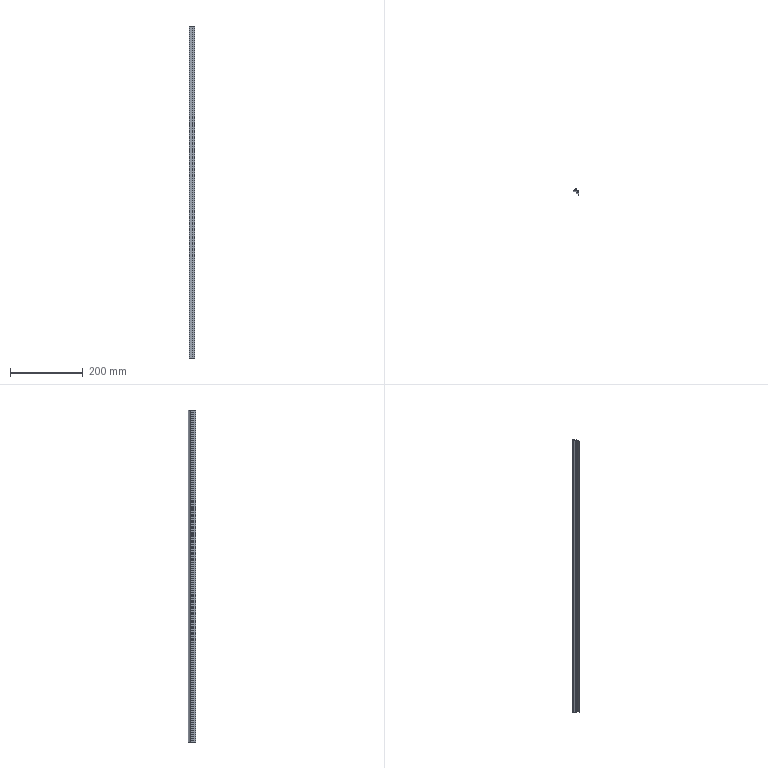Part | SolidWorks | features BaseBody 1, ICE 1, MoveFace 1 | 1 solid | 27 faces | box 14 x 20.3 x 915 mm | volume 46588 mm3 | plane 20 | cylinder 7 | commonest cylinder face diameters 0.387 x2 0.8 x2 0.4 x1 20 x1 22 x1
STEP:
#1=CARTESIAN_POINT('',(-5.304,-0.625,200.));
#2=VERTEX_POINT('',#1);
#3=CARTESIAN_POINT('',(-5.449,-0.8125,200.));
#4=VERTEX_POINT('',#3);
#5=CARTESIAN_POINT('',(-5.255,-0.8125,200.));
#6=DIRECTION('',(0.,0.,1.));
#7=DIRECTION('',(-1.,0.,0.));
#8=AXIS2_PLACEMENT_3D('',#5,#6,#7);
#9=CIRCLE('',#8,0.1937);
#10=EDGE_CURVE('',#2,#4,#9,.T.);
#11=ORIENTED_EDGE('',*,*,#10,.T.);
#12=CARTESIAN_POINT('',(-5.449,-0.8125,-715.));
#13=VERTEX_POINT('',#12);
#14=CARTESIAN_POINT('',(-5.449,-0.8125,230.));
#15=DIRECTION('',(0.,0.,-1.));
#16=VECTOR('',#15,1000.);
#17=LINE('',#14,#16);
#18=EDGE_CURVE('',#4,#13,#17,.T.);
#19=ORIENTED_EDGE('',*,*,#18,.T.);
#20=CARTESIAN_POINT('',(-5.304,-0.625,-715.));
#21=VERTEX_POINT('',#20);
#22=CARTESIAN_POINT('',(-5.255,-0.8125,-715.));
#23=DIRECTION('',(0.,0.,-1.));
#24=DIRECTION('',(1.,0.,0.));
#25=AXIS2_PLACEMENT_3D('',#22,#23,#24);
#26=CIRCLE('',#25,0.1937);
#27=EDGE_CURVE('',#13,#21,#26,.T.);
#28=ORIENTED_EDGE('',*,*,#27,.T.);
#29=CARTESIAN_POINT('',(-5.304,-0.625,230.));
#30=DIRECTION('',(0.,0.,-1.));
#31=VECTOR('',#30,1000.);
#32=LINE('',#29,#31);
#33=EDGE_CURVE('',#2,#21,#32,.T.);
#34=ORIENTED_EDGE('',*,*,#33,.F.);
#35=EDGE_LOOP('',(#11,#19,#28,#34));
#36=FACE_OUTER_BOUND('',#35,.T.);
#37=CARTESIAN_POINT('',(-5.255,-0.8125,230.));
#38=DIRECTION('',(0.,0.,-1.));
#39=DIRECTION('',(-1.,0.,0.));
#40=AXIS2_PLACEMENT_3D('',#37,#38,#39);
#41=CYLINDRICAL_SURFACE('',#40,0.1937);
#42=ADVANCED_FACE('',(#36),#41,.F.);
#43=CARTESIAN_POINT('',(5.,-1.,-715.));
#44=VERTEX_POINT('',#43);
#45=CARTESIAN_POINT('',(5.,-14.3,-715.));
#46=VERTEX_POINT('',#45);
#47=CARTESIAN_POINT('',(5.,29.623,-715.));
#48=DIRECTION('',(0.,-1.,0.));
#49=VECTOR('',#48,1000.);
#50=LINE('',#47,#49);
#51=EDGE_CURVE('',#44,#46,#50,.T.);
#52=ORIENTED_EDGE('',*,*,#51,.F.);
#53=CARTESIAN_POINT('',(5.,-1.,200.));
#54=VERTEX_POINT('',#53);
#55=CARTESIAN_POINT('',(5.,-1.,230.));
#56=DIRECTION('',(0.,0.,-1.));
#57=VECTOR('',#56,1000.);
#58=LINE('',#55,#57);
#59=EDGE_CURVE('',#54,#44,#58,.T.);
#60=ORIENTED_EDGE('',*,*,#59,.F.);
#61=CARTESIAN_POINT('',(5.,-14.3,200.));
#62=VERTEX_POINT('',#61);
#63=CARTESIAN_POINT('',(5.,-14.3,200.));
#64=DIRECTION('',(0.,1.,0.));
#65=VECTOR('',#64,1000.);
#66=LINE('',#63,#65);
#67=EDGE_CURVE('',#62,#54,#66,.T.);
#68=ORIENTED_EDGE('',*,*,#67,.F.);
#69=CARTESIAN_POINT('',(5.,-14.3,230.));
#70=DIRECTION('',(0.,0.,1.));
#71=VECTOR('',#70,1000.);
#72=LINE('',#69,#71);
#73=EDGE_CURVE('',#46,#62,#72,.T.);
#74=ORIENTED_EDGE('',*,*,#73,.F.);
#75=EDGE_LOOP('',(#52,#60,#68,#74));
#76=FACE_OUTER_BOUND('',#75,.T.);
#77=CARTESIAN_POINT('',(5.,-14.3,230.));
#78=DIRECTION('',(-1.,0.,0.));
#79=DIRECTION('',(0.,0.,1.));
#80=AXIS2_PLACEMENT_3D('',#77,#78,#79);
#81=PLANE('',#80);
#82=ADVANCED_FACE('',(#76),#81,.F.);
#83=CARTESIAN_POINT('',(-9.,-2.,-715.));
#84=VERTEX_POINT('',#83);
#85=CARTESIAN_POINT('',(-9.,-2.,200.));
#86=VERTEX_POINT('',#85);
#87=CARTESIAN_POINT('',(-9.,-2.,230.));
#88=DIRECTION('',(0.,0.,1.));
#89=VECTOR('',#88,1000.);
#90=LINE('',#87,#89);
#91=EDGE_CURVE('',#84,#86,#90,.T.);
#92=ORIENTED_EDGE('',*,*,#91,.F.);
#93=CARTESIAN_POINT('',(0.9,-2.,-715.));
#94=VERTEX_POINT('',#93);
#95=CARTESIAN_POINT('',(5.,-2.,-715.));
#96=DIRECTION('',(-1.,0.,0.));
#97=VECTOR('',#96,1000.);
#98=LINE('',#95,#97);
#99=EDGE_CURVE('',#94,#84,#98,.T.);
#100=ORIENTED_EDGE('',*,*,#99,.F.);
#101=CARTESIAN_POINT('',(0.9,-2.,200.));
#102=VERTEX_POINT('',#101);
#103=CARTESIAN_POINT('',(0.9,-2.,230.));
#104=DIRECTION('',(0.,0.,-1.));
#105=VECTOR('',#104,1000.);
#106=LINE('',#103,#105);
#107=EDGE_CURVE('',#102,#94,#106,.T.);
#108=ORIENTED_EDGE('',*,*,#107,.F.);
#109=CARTESIAN_POINT('',(5.,-2.,200.));
#110=DIRECTION('',(1.,0.,0.));
#111=VECTOR('',#110,1000.);
#112=LINE('',#109,#111);
#113=EDGE_CURVE('',#86,#102,#112,.T.);
#114=ORIENTED_EDGE('',*,*,#113,.F.);
#115=EDGE_LOOP('',(#92,#100,#108,#114));
#116=FACE_OUTER_BOUND('',#115,.T.);
#117=CARTESIAN_POINT('',(-9.,-2.,230.));
#118=DIRECTION('',(0.,1.,0.));
#119=DIRECTION('',(0.,0.,1.));
#120=AXIS2_PLACEMENT_3D('',#117,#118,#119);
#121=PLANE('',#120);
#122=ADVANCED_FACE('',(#116),#121,.F.);
#123=CARTESIAN_POINT('',(4.,-6.,200.));
#124=VERTEX_POINT('',#123);
#125=CARTESIAN_POINT('',(4.,-3.,200.));
#126=VERTEX_POINT('',#125);
#127=CARTESIAN_POINT('',(4.,29.623,200.));
#128=DIRECTION('',(0.,1.,0.));
#129=VECTOR('',#128,1000.);
#130=LINE('',#127,#129);
#131=EDGE_CURVE('',#124,#126,#130,.T.);
#132=ORIENTED_EDGE('',*,*,#131,.F.);
#133=CARTESIAN_POINT('',(1.,-6.,200.));
#134=VERTEX_POINT('',#133);
#135=CARTESIAN_POINT('',(5.,-6.,200.));
#136=DIRECTION('',(1.,0.,0.));
#137=VECTOR('',#136,1000.);
#138=LINE('',#135,#137);
#139=EDGE_CURVE('',#134,#124,#138,.T.);
#140=ORIENTED_EDGE('',*,*,#139,.F.);
#141=CARTESIAN_POINT('',(1.,-6.7,200.));
#142=VERTEX_POINT('',#141);
#143=CARTESIAN_POINT('',(1.,-6.,200.));
#144=DIRECTION('',(0.,-1.,0.));
#145=VECTOR('',#144,1000.);
#146=LINE('',#143,#145);
#147=EDGE_CURVE('',#134,#142,#146,.T.);
#148=ORIENTED_EDGE('',*,*,#147,.T.);
#149=CARTESIAN_POINT('',(-1.7,-6.7,200.));
#150=VERTEX_POINT('',#149);
#151=CARTESIAN_POINT('',(5.,-6.7,200.));
#152=DIRECTION('',(1.,0.,0.));
#153=VECTOR('',#152,1000.);
#154=LINE('',#151,#153);
#155=EDGE_CURVE('',#150,#142,#154,.T.);
#156=ORIENTED_EDGE('',*,*,#155,.F.);
#157=CARTESIAN_POINT('',(-1.7,-7.7,200.));
#158=VERTEX_POINT('',#157);
#159=CARTESIAN_POINT('',(-1.7,-6.7,200.));
#160=DIRECTION('',(0.,-1.,0.));
#161=VECTOR('',#160,1000.);
#162=LINE('',#159,#161);
#163=EDGE_CURVE('',#150,#158,#162,.T.);
#164=ORIENTED_EDGE('',*,*,#163,.T.);
#165=CARTESIAN_POINT('',(4.,-7.7,200.));
#166=VERTEX_POINT('',#165);
#167=CARTESIAN_POINT('',(5.,-7.7,200.));
#168=DIRECTION('',(-1.,0.,0.));
#169=VECTOR('',#168,1000.);
#170=LINE('',#167,#169);
#171=EDGE_CURVE('',#166,#158,#170,.T.);
#172=ORIENTED_EDGE('',*,*,#171,.F.);
#173=CARTESIAN_POINT('',(4.,-14.3,200.));
#174=VERTEX_POINT('',#173);
#175=CARTESIAN_POINT('',(4.,29.623,200.));
#176=DIRECTION('',(0.,1.,0.));
#177=VECTOR('',#176,1000.);
#178=LINE('',#175,#177);
#179=EDGE_CURVE('',#174,#166,#178,.T.);
#180=ORIENTED_EDGE('',*,*,#179,.F.);
#181=CARTESIAN_POINT('',(5.,-14.3,200.));
#182=DIRECTION('',(-1.,0.,0.));
#183=VECTOR('',#182,1000.);
#184=LINE('',#181,#183);
#185=EDGE_CURVE('',#62,#174,#184,.T.);
#186=ORIENTED_EDGE('',*,*,#185,.F.);
#187=ORIENTED_EDGE('',*,*,#67,.T.);
#188=CARTESIAN_POINT('',(-5.207,-1.,200.));
#189=VERTEX_POINT('',#188);
#190=CARTESIAN_POINT('',(5.,-1.,200.));
#191=DIRECTION('',(1.,0.,0.));
#192=VECTOR('',#191,1000.);
#193=LINE('',#190,#192);
#194=EDGE_CURVE('',#189,#54,#193,.T.);
#195=ORIENTED_EDGE('',*,*,#194,.F.);
#196=CARTESIAN_POINT('',(-5.255,-0.8125,200.));
#197=DIRECTION('',(0.,0.,1.));
#198=DIRECTION('',(-1.,0.,0.));
#199=AXIS2_PLACEMENT_3D('',#196,#197,#198);
#200=CIRCLE('',#199,0.1937);
#201=EDGE_CURVE('',#4,#189,#200,.T.);
#202=ORIENTED_EDGE('',*,*,#201,.F.);
#203=ORIENTED_EDGE('',*,*,#10,.F.);
#204=CARTESIAN_POINT('',(-1.368,3.063,200.));
#205=VERTEX_POINT('',#204);
#206=CARTESIAN_POINT('',(-10.628,9.,200.));
#207=DIRECTION('',(0.,0.,1.));
#208=DIRECTION('',(-1.,0.,0.));
#209=AXIS2_PLACEMENT_3D('',#206,#207,#208);
#210=CIRCLE('',#209,11.);
#211=EDGE_CURVE('',#2,#205,#210,.T.);
#212=ORIENTED_EDGE('',*,*,#211,.T.);
#213=CARTESIAN_POINT('',(-1.,2.955,200.));
#214=VERTEX_POINT('',#213);
#215=CARTESIAN_POINT('',(-1.2,2.955,200.));
#216=DIRECTION('',(0.,0.,1.));
#217=DIRECTION('',(-1.,0.,0.));
#218=AXIS2_PLACEMENT_3D('',#215,#216,#217);
#219=CIRCLE('',#218,0.2);
#220=EDGE_CURVE('',#214,#205,#219,.T.);
#221=ORIENTED_EDGE('',*,*,#220,.F.);
#222=CARTESIAN_POINT('',(-1.,1.5,200.));
#223=VERTEX_POINT('',#222);
#224=CARTESIAN_POINT('',(-1.,2.955,200.));
#225=DIRECTION('',(0.,1.,0.));
#226=VECTOR('',#225,1000.);
#227=LINE('',#224,#226);
#228=EDGE_CURVE('',#223,#214,#227,.T.);
#229=ORIENTED_EDGE('',*,*,#228,.F.);
#230=CARTESIAN_POINT('',(0.,1.5,200.));
#231=VERTEX_POINT('',#230);
#232=CARTESIAN_POINT('',(-1.,1.5,200.));
#233=DIRECTION('',(-1.,0.,0.));
#234=VECTOR('',#233,1000.);
#235=LINE('',#232,#234);
#236=EDGE_CURVE('',#231,#223,#235,.T.);
#237=ORIENTED_EDGE('',*,*,#236,.F.);
#238=CARTESIAN_POINT('',(0.,6.,200.));
#239=VERTEX_POINT('',#238);
#240=CARTESIAN_POINT('',(0.,1.5,200.));
#241=DIRECTION('',(0.,-1.,0.));
#242=VECTOR('',#241,1000.);
#243=LINE('',#240,#242);
#244=EDGE_CURVE('',#239,#231,#243,.T.);
#245=ORIENTED_EDGE('',*,*,#244,.F.);
#246=CARTESIAN_POINT('',(-0.8,6.,200.));
#247=VERTEX_POINT('',#246);
#248=CARTESIAN_POINT('',(0.,6.,200.));
#249=DIRECTION('',(1.,0.,0.));
#250=VECTOR('',#249,1000.);
#251=LINE('',#248,#250);
#252=EDGE_CURVE('',#247,#239,#251,.T.);
#253=ORIENTED_EDGE('',*,*,#252,.F.);
#254=CARTESIAN_POINT('',(-1.178,5.731,200.));
#255=VERTEX_POINT('',#254);
#256=CARTESIAN_POINT('',(-0.8,5.6,200.));
#257=DIRECTION('',(0.,0.,1.));
#258=DIRECTION('',(-1.,0.,0.));
#259=AXIS2_PLACEMENT_3D('',#256,#257,#258);
#260=CIRCLE('',#259,0.4);
#261=EDGE_CURVE('',#247,#255,#260,.T.);
#262=ORIENTED_EDGE('',*,*,#261,.T.);
#263=CARTESIAN_POINT('',(-8.678,-0.8077,200.));
#264=VERTEX_POINT('',#263);
#265=CARTESIAN_POINT('',(-10.628,9.,200.));
#266=DIRECTION('',(0.,0.,1.));
#267=DIRECTION('',(-1.,0.,0.));
#268=AXIS2_PLACEMENT_3D('',#265,#266,#267);
#269=CIRCLE('',#268,10.);
#270=EDGE_CURVE('',#264,#255,#269,.T.);
#271=ORIENTED_EDGE('',*,*,#270,.F.);
#272=CARTESIAN_POINT('',(-9.,-1.2,200.));
#273=VERTEX_POINT('',#272);
#274=CARTESIAN_POINT('',(-8.6,-1.2,200.));
#275=DIRECTION('',(0.,0.,1.));
#276=DIRECTION('',(-1.,0.,0.));
#277=AXIS2_PLACEMENT_3D('',#274,#275,#276);
#278=CIRCLE('',#277,0.4);
#279=EDGE_CURVE('',#264,#273,#278,.T.);
#280=ORIENTED_EDGE('',*,*,#279,.T.);
#281=CARTESIAN_POINT('',(-9.,8.,200.));
#282=DIRECTION('',(0.,-1.,0.));
#283=VECTOR('',#282,1000.);
#284=LINE('',#281,#283);
#285=EDGE_CURVE('',#273,#86,#284,.T.);
#286=ORIENTED_EDGE('',*,*,#285,.T.);
#287=ORIENTED_EDGE('',*,*,#113,.T.);
#288=CARTESIAN_POINT('',(0.9,-3.,200.));
#289=VERTEX_POINT('',#288);
#290=CARTESIAN_POINT('',(0.9,29.623,200.));
#291=DIRECTION('',(0.,1.,0.));
#292=VECTOR('',#291,1000.);
#293=LINE('',#290,#292);
#294=EDGE_CURVE('',#289,#102,#293,.T.);
#295=ORIENTED_EDGE('',*,*,#294,.F.);
#296=CARTESIAN_POINT('',(5.,-3.,200.));
#297=DIRECTION('',(-1.,0.,0.));
#298=VECTOR('',#297,1000.);
#299=LINE('',#296,#298);
#300=EDGE_CURVE('',#126,#289,#299,.T.);
#301=ORIENTED_EDGE('',*,*,#300,.F.);
#302=EDGE_LOOP('',(#132,#140,#148,#156,#164,#172,#180,#186,#187,#195,#202,#203,#212,#221,#229,#237,#245,#253,#262,#271,#280,#286,#287,#295,#301));
#303=FACE_OUTER_BOUND('',#302,.T.);
#304=CARTESIAN_POINT('',(5.,29.623,200.));
#305=DIRECTION('',(0.,0.,-1.));
#306=DIRECTION('',(-1.,0.,0.));
#307=AXIS2_PLACEMENT_3D('',#304,#305,#306);
#308=PLANE('',#307);
#309=ADVANCED_FACE('',(#303),#308,.F.);
#310=ORIENTED_EDGE('',*,*,#185,.T.);
#311=CARTESIAN_POINT('',(4.,-14.3,-715.));
#312=VERTEX_POINT('',#311);
#313=CARTESIAN_POINT('',(4.,-14.3,230.));
#314=DIRECTION('',(0.,0.,1.));
#315=VECTOR('',#314,1000.);
#316=LINE('',#313,#315);
#317=EDGE_CURVE('',#312,#174,#316,.T.);
#318=ORIENTED_EDGE('',*,*,#317,.F.);
#319=CARTESIAN_POINT('',(5.,-14.3,-715.));
#320=DIRECTION('',(-1.,0.,0.));
#321=VECTOR('',#320,1000.);
#322=LINE('',#319,#321);
#323=EDGE_CURVE('',#46,#312,#322,.T.);
#324=ORIENTED_EDGE('',*,*,#323,.F.);
#325=ORIENTED_EDGE('',*,*,#73,.T.);
#326=EDGE_LOOP('',(#310,#318,#324,#325));
#327=FACE_OUTER_BOUND('',#326,.T.);
#328=CARTESIAN_POINT('',(4.,-14.3,230.));
#329=DIRECTION('',(0.,1.,0.));
#330=DIRECTION('',(0.,0.,1.));
#331=AXIS2_PLACEMENT_3D('',#328,#329,#330);
#332=PLANE('',#331);
#333=ADVANCED_FACE('',(#327),#332,.F.);
#334=ORIENTED_EDGE('',*,*,#51,.T.);
#335=ORIENTED_EDGE('',*,*,#323,.T.);
#336=CARTESIAN_POINT('',(4.,-7.7,-715.));
#337=VERTEX_POINT('',#336);
#338=CARTESIAN_POINT('',(4.,-7.7,-715.));
#339=DIRECTION('',(0.,-1.,0.));
#340=VECTOR('',#339,1000.);
#341=LINE('',#338,#340);
#342=EDGE_CURVE('',#337,#312,#341,.T.);
#343=ORIENTED_EDGE('',*,*,#342,.F.);
#344=CARTESIAN_POINT('',(-1.7,-7.7,-715.));
#345=VERTEX_POINT('',#344);
#346=CARTESIAN_POINT('',(-1.7,-7.7,-715.));
#347=DIRECTION('',(1.,0.,0.));
#348=VECTOR('',#347,1000.);
#349=LINE('',#346,#348);
#350=EDGE_CURVE('',#345,#337,#349,.T.);
#351=ORIENTED_EDGE('',*,*,#350,.F.);
#352=CARTESIAN_POINT('',(-1.7,-6.7,-715.));
#353=VERTEX_POINT('',#352);
#354=CARTESIAN_POINT('',(-1.7,29.623,-715.));
#355=DIRECTION('',(0.,1.,0.));
#356=VECTOR('',#355,1000.);
#357=LINE('',#354,#356);
#358=EDGE_CURVE('',#345,#353,#357,.T.);
#359=ORIENTED_EDGE('',*,*,#358,.T.);
#360=CARTESIAN_POINT('',(1.,-6.7,-715.));
#361=VERTEX_POINT('',#360);
#362=CARTESIAN_POINT('',(1.,-6.7,-715.));
#363=DIRECTION('',(-1.,0.,0.));
#364=VECTOR('',#363,1000.);
#365=LINE('',#362,#364);
#366=EDGE_CURVE('',#361,#353,#365,.T.);
#367=ORIENTED_EDGE('',*,*,#366,.F.);
#368=CARTESIAN_POINT('',(1.,-6.,-715.));
#369=VERTEX_POINT('',#368);
#370=CARTESIAN_POINT('',(1.,29.623,-715.));
#371=DIRECTION('',(0.,1.,0.));
#372=VECTOR('',#371,1000.);
#373=LINE('',#370,#372);
#374=EDGE_CURVE('',#361,#369,#373,.T.);
#375=ORIENTED_EDGE('',*,*,#374,.T.);
#376=CARTESIAN_POINT('',(4.,-6.,-715.));
#377=VERTEX_POINT('',#376);
#378=CARTESIAN_POINT('',(4.,-6.,-715.));
#379=DIRECTION('',(-1.,0.,0.));
#380=VECTOR('',#379,1000.);
#381=LINE('',#378,#380);
#382=EDGE_CURVE('',#377,#369,#381,.T.);
#383=ORIENTED_EDGE('',*,*,#382,.F.);
#384=CARTESIAN_POINT('',(4.,-3.,-715.));
#385=VERTEX_POINT('',#384);
#386=CARTESIAN_POINT('',(4.,-3.,-715.));
#387=DIRECTION('',(0.,-1.,0.));
#388=VECTOR('',#387,1000.);
#389=LINE('',#386,#388);
#390=EDGE_CURVE('',#385,#377,#389,.T.);
#391=ORIENTED_EDGE('',*,*,#390,.F.);
#392=CARTESIAN_POINT('',(0.9,-3.,-715.));
#393=VERTEX_POINT('',#392);
#394=CARTESIAN_POINT('',(0.9,-3.,-715.));
#395=DIRECTION('',(1.,0.,0.));
#396=VECTOR('',#395,1000.);
#397=LINE('',#394,#396);
#398=EDGE_CURVE('',#393,#385,#397,.T.);
#399=ORIENTED_EDGE('',*,*,#398,.F.);
#400=CARTESIAN_POINT('',(0.9,-2.,-715.));
#401=DIRECTION('',(0.,-1.,0.));
#402=VECTOR('',#401,1000.);
#403=LINE('',#400,#402);
#404=EDGE_CURVE('',#94,#393,#403,.T.);
#405=ORIENTED_EDGE('',*,*,#404,.F.);
#406=ORIENTED_EDGE('',*,*,#99,.T.);
#407=CARTESIAN_POINT('',(-9.,-1.2,-715.));
#408=VERTEX_POINT('',#407);
#409=CARTESIAN_POINT('',(-9.,-1.2,-715.));
#410=DIRECTION('',(0.,-1.,0.));
#411=VECTOR('',#410,1000.);
#412=LINE('',#409,#411);
#413=EDGE_CURVE('',#408,#84,#412,.T.);
#414=ORIENTED_EDGE('',*,*,#413,.F.);
#415=CARTESIAN_POINT('',(-8.678,-0.8077,-715.));
#416=VERTEX_POINT('',#415);
#417=CARTESIAN_POINT('',(-8.6,-1.2,-715.));
#418=DIRECTION('',(0.,0.,-1.));
#419=DIRECTION('',(1.,0.,0.));
#420=AXIS2_PLACEMENT_3D('',#417,#418,#419);
#421=CIRCLE('',#420,0.4);
#422=EDGE_CURVE('',#408,#416,#421,.T.);
#423=ORIENTED_EDGE('',*,*,#422,.T.);
#424=CARTESIAN_POINT('',(-1.178,5.731,-715.));
#425=VERTEX_POINT('',#424);
#426=CARTESIAN_POINT('',(-10.628,9.,-715.));
#427=DIRECTION('',(0.,0.,-1.));
#428=DIRECTION('',(1.,0.,0.));
#429=AXIS2_PLACEMENT_3D('',#426,#427,#428);
#430=CIRCLE('',#429,10.);
#431=EDGE_CURVE('',#425,#416,#430,.T.);
#432=ORIENTED_EDGE('',*,*,#431,.F.);
#433=CARTESIAN_POINT('',(-0.8,6.,-715.));
#434=VERTEX_POINT('',#433);
#435=CARTESIAN_POINT('',(-0.8,5.6,-715.));
#436=DIRECTION('',(0.,0.,-1.));
#437=DIRECTION('',(1.,0.,0.));
#438=AXIS2_PLACEMENT_3D('',#435,#436,#437);
#439=CIRCLE('',#438,0.4);
#440=EDGE_CURVE('',#425,#434,#439,.T.);
#441=ORIENTED_EDGE('',*,*,#440,.T.);
#442=CARTESIAN_POINT('',(0.,6.,-715.));
#443=VERTEX_POINT('',#442);
#444=CARTESIAN_POINT('',(0.,6.,-715.));
#445=DIRECTION('',(-1.,0.,0.));
#446=VECTOR('',#445,1000.);
#447=LINE('',#444,#446);
#448=EDGE_CURVE('',#443,#434,#447,.T.);
#449=ORIENTED_EDGE('',*,*,#448,.F.);
#450=CARTESIAN_POINT('',(0.,1.5,-715.));
#451=VERTEX_POINT('',#450);
#452=CARTESIAN_POINT('',(0.,1.5,-715.));
#453=DIRECTION('',(0.,1.,0.));
#454=VECTOR('',#453,1000.);
#455=LINE('',#452,#454);
#456=EDGE_CURVE('',#451,#443,#455,.T.);
#457=ORIENTED_EDGE('',*,*,#456,.F.);
#458=CARTESIAN_POINT('',(-1.,1.5,-715.));
#459=VERTEX_POINT('',#458);
#460=CARTESIAN_POINT('',(-1.,1.5,-715.));
#461=DIRECTION('',(1.,0.,0.));
#462=VECTOR('',#461,1000.);
#463=LINE('',#460,#462);
#464=EDGE_CURVE('',#459,#451,#463,.T.);
#465=ORIENTED_EDGE('',*,*,#464,.F.);
#466=CARTESIAN_POINT('',(-1.,2.955,-715.));
#467=VERTEX_POINT('',#466);
#468=CARTESIAN_POINT('',(-1.,2.955,-715.));
#469=DIRECTION('',(0.,-1.,0.));
#470=VECTOR('',#469,1000.);
#471=LINE('',#468,#470);
#472=EDGE_CURVE('',#467,#459,#471,.T.);
#473=ORIENTED_EDGE('',*,*,#472,.F.);
#474=CARTESIAN_POINT('',(-1.368,3.063,-715.));
#475=VERTEX_POINT('',#474);
#476=CARTESIAN_POINT('',(-1.2,2.955,-715.));
#477=DIRECTION('',(0.,0.,-1.));
#478=DIRECTION('',(1.,0.,0.));
#479=AXIS2_PLACEMENT_3D('',#476,#477,#478);
#480=CIRCLE('',#479,0.2);
#481=EDGE_CURVE('',#475,#467,#480,.T.);
#482=ORIENTED_EDGE('',*,*,#481,.F.);
#483=CARTESIAN_POINT('',(-10.628,9.,-715.));
#484=DIRECTION('',(0.,0.,-1.));
#485=DIRECTION('',(1.,0.,0.));
#486=AXIS2_PLACEMENT_3D('',#483,#484,#485);
#487=CIRCLE('',#486,11.);
#488=EDGE_CURVE('',#475,#21,#487,.T.);
#489=ORIENTED_EDGE('',*,*,#488,.T.);
#490=ORIENTED_EDGE('',*,*,#27,.F.);
#491=CARTESIAN_POINT('',(-5.207,-1.,-715.));
#492=VERTEX_POINT('',#491);
#493=CARTESIAN_POINT('',(-5.255,-0.8125,-715.));
#494=DIRECTION('',(0.,0.,-1.));
#495=DIRECTION('',(1.,0.,0.));
#496=AXIS2_PLACEMENT_3D('',#493,#494,#495);
#497=CIRCLE('',#496,0.1937);
#498=EDGE_CURVE('',#492,#13,#497,.T.);
#499=ORIENTED_EDGE('',*,*,#498,.F.);
#500=CARTESIAN_POINT('',(5.,-1.,-715.));
#501=DIRECTION('',(-1.,0.,0.));
#502=VECTOR('',#501,1000.);
#503=LINE('',#500,#502);
#504=EDGE_CURVE('',#44,#492,#503,.T.);
#505=ORIENTED_EDGE('',*,*,#504,.F.);
#506=EDGE_LOOP('',(#334,#335,#343,#351,#359,#367,#375,#383,#391,#399,#405,#406,#414,#423,#432,#441,#449,#457,#465,#473,#482,#489,#490,#499,#505));
#507=FACE_OUTER_BOUND('',#506,.T.);
#508=CARTESIAN_POINT('',(5.,29.623,-715.));
#509=DIRECTION('',(0.,0.,1.));
#510=DIRECTION('',(1.,0.,0.));
#511=AXIS2_PLACEMENT_3D('',#508,#509,#510);
#512=PLANE('',#511);
#513=ADVANCED_FACE('',(#507),#512,.F.);
#514=ORIENTED_EDGE('',*,*,#59,.T.);
#515=ORIENTED_EDGE('',*,*,#504,.T.);
#516=CARTESIAN_POINT('',(-5.207,-1.,230.));
#517=DIRECTION('',(0.,0.,-1.));
#518=VECTOR('',#517,1000.);
#519=LINE('',#516,#518);
#520=EDGE_CURVE('',#189,#492,#519,.T.);
#521=ORIENTED_EDGE('',*,*,#520,.F.);
#522=ORIENTED_EDGE('',*,*,#194,.T.);
#523=EDGE_LOOP('',(#514,#515,#521,#522));
#524=FACE_OUTER_BOUND('',#523,.T.);
#525=CARTESIAN_POINT('',(5.,-1.,230.));
#526=DIRECTION('',(0.,-1.,0.));
#527=DIRECTION('',(0.,0.,-1.));
#528=AXIS2_PLACEMENT_3D('',#525,#526,#527);
#529=PLANE('',#528);
#530=ADVANCED_FACE('',(#524),#529,.F.);
#531=CARTESIAN_POINT('',(-9.,-1.2,230.));
#532=DIRECTION('',(0.,0.,1.));
#533=VECTOR('',#532,1000.);
#534=LINE('',#531,#533);
#535=EDGE_CURVE('',#408,#273,#534,.T.);
#536=ORIENTED_EDGE('',*,*,#535,.F.);
#537=ORIENTED_EDGE('',*,*,#413,.T.);
#538=ORIENTED_EDGE('',*,*,#91,.T.);
#539=ORIENTED_EDGE('',*,*,#285,.F.);
#540=EDGE_LOOP('',(#536,#537,#538,#539));
#541=FACE_OUTER_BOUND('',#540,.T.);
#542=CARTESIAN_POINT('',(-9.,-1.2,230.));
#543=DIRECTION('',(1.,0.,0.));
#544=DIRECTION('',(0.,0.,-1.));
#545=AXIS2_PLACEMENT_3D('',#542,#543,#544);
#546=PLANE('',#545);
#547=ADVANCED_FACE('',(#541),#546,.F.);
#548=ORIENTED_EDGE('',*,*,#294,.T.);
#549=ORIENTED_EDGE('',*,*,#107,.T.);
#550=ORIENTED_EDGE('',*,*,#404,.T.);
#551=CARTESIAN_POINT('',(0.9,-3.,230.));
#552=DIRECTION('',(0.,0.,-1.));
#553=VECTOR('',#552,1000.);
#554=LINE('',#551,#553);
#555=EDGE_CURVE('',#289,#393,#554,.T.);
#556=ORIENTED_EDGE('',*,*,#555,.F.);
#557=EDGE_LOOP('',(#548,#549,#550,#556));
#558=FACE_OUTER_BOUND('',#557,.T.);
#559=CARTESIAN_POINT('',(0.9,-2.,230.));
#560=DIRECTION('',(1.,0.,0.));
#561=DIRECTION('',(0.,0.,-1.));
#562=AXIS2_PLACEMENT_3D('',#559,#560,#561);
#563=PLANE('',#562);
#564=ADVANCED_FACE('',(#558),#563,.F.);
#565=ORIENTED_EDGE('',*,*,#300,.T.);
#566=ORIENTED_EDGE('',*,*,#555,.T.);
#567=ORIENTED_EDGE('',*,*,#398,.T.);
#568=CARTESIAN_POINT('',(4.,-3.,230.));
#569=DIRECTION('',(0.,0.,-1.));
#570=VECTOR('',#569,1000.);
#571=LINE('',#568,#570);
#572=EDGE_CURVE('',#126,#385,#571,.T.);
#573=ORIENTED_EDGE('',*,*,#572,.F.);
#574=EDGE_LOOP('',(#565,#566,#567,#573));
#575=FACE_OUTER_BOUND('',#574,.T.);
#576=CARTESIAN_POINT('',(0.9,-3.,230.));
#577=DIRECTION('',(0.,1.,0.));
#578=DIRECTION('',(0.,0.,1.));
#579=AXIS2_PLACEMENT_3D('',#576,#577,#578);
#580=PLANE('',#579);
#581=ADVANCED_FACE('',(#575),#580,.F.);
#582=ORIENTED_EDGE('',*,*,#131,.T.);
#583=ORIENTED_EDGE('',*,*,#572,.T.);
#584=ORIENTED_EDGE('',*,*,#390,.T.);
#585=CARTESIAN_POINT('',(4.,-6.,230.));
#586=DIRECTION('',(0.,0.,-1.));
#587=VECTOR('',#586,1000.);
#588=LINE('',#585,#587);
#589=EDGE_CURVE('',#124,#377,#588,.T.);
#590=ORIENTED_EDGE('',*,*,#589,.F.);
#591=EDGE_LOOP('',(#582,#583,#584,#590));
#592=FACE_OUTER_BOUND('',#591,.T.);
#593=CARTESIAN_POINT('',(4.,-3.,230.));
#594=DIRECTION('',(1.,0.,0.));
#595=DIRECTION('',(0.,0.,-1.));
#596=AXIS2_PLACEMENT_3D('',#593,#594,#595);
#597=PLANE('',#596);
#598=ADVANCED_FACE('',(#592),#597,.F.);
#599=ORIENTED_EDGE('',*,*,#139,.T.);
#600=ORIENTED_EDGE('',*,*,#589,.T.);
#601=ORIENTED_EDGE('',*,*,#382,.T.);
#602=CARTESIAN_POINT('',(1.,-6.,230.));
#603=DIRECTION('',(0.,0.,-1.));
#604=VECTOR('',#603,1000.);
#605=LINE('',#602,#604);
#606=EDGE_CURVE('',#134,#369,#605,.T.);
#607=ORIENTED_EDGE('',*,*,#606,.F.);
#608=EDGE_LOOP('',(#599,#600,#601,#607));
#609=FACE_OUTER_BOUND('',#608,.T.);
#610=CARTESIAN_POINT('',(4.,-6.,230.));
#611=DIRECTION('',(0.,-1.,0.));
#612=DIRECTION('',(0.,0.,-1.));
#613=AXIS2_PLACEMENT_3D('',#610,#611,#612);
#614=PLANE('',#613);
#615=ADVANCED_FACE('',(#609),#614,.F.);
#616=ORIENTED_EDGE('',*,*,#155,.T.);
#617=CARTESIAN_POINT('',(1.,-6.7,230.));
#618=DIRECTION('',(0.,0.,1.));
#619=VECTOR('',#618,1000.);
#620=LINE('',#617,#619);
#621=EDGE_CURVE('',#361,#142,#620,.T.);
#622=ORIENTED_EDGE('',*,*,#621,.F.);
#623=ORIENTED_EDGE('',*,*,#366,.T.);
#624=CARTESIAN_POINT('',(-1.7,-6.7,230.));
#625=DIRECTION('',(0.,0.,-1.));
#626=VECTOR('',#625,1000.);
#627=LINE('',#624,#626);
#628=EDGE_CURVE('',#150,#353,#627,.T.);
#629=ORIENTED_EDGE('',*,*,#628,.F.);
#630=EDGE_LOOP('',(#616,#622,#623,#629));
#631=FACE_OUTER_BOUND('',#630,.T.);
#632=CARTESIAN_POINT('',(1.,-6.7,230.));
#633=DIRECTION('',(0.,-1.,0.));
#634=DIRECTION('',(0.,0.,-1.));
#635=AXIS2_PLACEMENT_3D('',#632,#633,#634);
#636=PLANE('',#635);
#637=ADVANCED_FACE('',(#631),#636,.F.);
#638=ORIENTED_EDGE('',*,*,#171,.T.);
#639=CARTESIAN_POINT('',(-1.7,-7.7,230.));
#640=DIRECTION('',(0.,0.,1.));
#641=VECTOR('',#640,1000.);
#642=LINE('',#639,#641);
#643=EDGE_CURVE('',#345,#158,#642,.T.);
#644=ORIENTED_EDGE('',*,*,#643,.F.);
#645=ORIENTED_EDGE('',*,*,#350,.T.);
#646=CARTESIAN_POINT('',(4.,-7.7,230.));
#647=DIRECTION('',(0.,0.,-1.));
#648=VECTOR('',#647,1000.);
#649=LINE('',#646,#648);
#650=EDGE_CURVE('',#166,#337,#649,.T.);
#651=ORIENTED_EDGE('',*,*,#650,.F.);
#652=EDGE_LOOP('',(#638,#644,#645,#651));
#653=FACE_OUTER_BOUND('',#652,.T.);
#654=CARTESIAN_POINT('',(-1.7,-7.7,230.));
#655=DIRECTION('',(0.,1.,0.));
#656=DIRECTION('',(0.,0.,1.));
#657=AXIS2_PLACEMENT_3D('',#654,#655,#656);
#658=PLANE('',#657);
#659=ADVANCED_FACE('',(#653),#658,.F.);
#660=ORIENTED_EDGE('',*,*,#179,.T.);
#661=ORIENTED_EDGE('',*,*,#650,.T.);
#662=ORIENTED_EDGE('',*,*,#342,.T.);
#663=ORIENTED_EDGE('',*,*,#317,.T.);
#664=EDGE_LOOP('',(#660,#661,#662,#663));
#665=FACE_OUTER_BOUND('',#664,.T.);
#666=CARTESIAN_POINT('',(4.,-7.7,230.));
#667=DIRECTION('',(1.,0.,0.));
#668=DIRECTION('',(0.,0.,-1.));
#669=AXIS2_PLACEMENT_3D('',#666,#667,#668);
#670=PLANE('',#669);
#671=ADVANCED_FACE('',(#665),#670,.F.);
#672=ORIENTED_EDGE('',*,*,#18,.F.);
#673=ORIENTED_EDGE('',*,*,#201,.T.);
#674=ORIENTED_EDGE('',*,*,#520,.T.);
#675=ORIENTED_EDGE('',*,*,#498,.T.);
#676=EDGE_LOOP('',(#672,#673,#674,#675));
#677=FACE_OUTER_BOUND('',#676,.T.);
#678=CARTESIAN_POINT('',(-5.255,-0.8125,230.));
#679=DIRECTION('',(0.,0.,-1.));
#680=DIRECTION('',(-1.,0.,0.));
#681=AXIS2_PLACEMENT_3D('',#678,#679,#680);
#682=CYLINDRICAL_SURFACE('',#681,0.1937);
#683=ADVANCED_FACE('',(#677),#682,.F.);
#684=CARTESIAN_POINT('',(-1.,2.955,230.));
#685=DIRECTION('',(0.,0.,1.));
#686=VECTOR('',#685,1000.);
#687=LINE('',#684,#686);
#688=EDGE_CURVE('',#467,#214,#687,.T.);
#689=ORIENTED_EDGE('',*,*,#688,.F.);
#690=ORIENTED_EDGE('',*,*,#472,.T.);
#691=CARTESIAN_POINT('',(-1.,1.5,230.));
#692=DIRECTION('',(0.,0.,-1.));
#693=VECTOR('',#692,1000.);
#694=LINE('',#691,#693);
#695=EDGE_CURVE('',#223,#459,#694,.T.);
#696=ORIENTED_EDGE('',*,*,#695,.F.);
#697=ORIENTED_EDGE('',*,*,#228,.T.);
#698=EDGE_LOOP('',(#689,#690,#696,#697));
#699=FACE_OUTER_BOUND('',#698,.T.);
#700=CARTESIAN_POINT('',(-1.,2.955,230.));
#701=DIRECTION('',(1.,0.,0.));
#702=DIRECTION('',(0.,0.,-1.));
#703=AXIS2_PLACEMENT_3D('',#700,#701,#702);
#704=PLANE('',#703);
#705=ADVANCED_FACE('',(#699),#704,.F.);
#706=ORIENTED_EDGE('',*,*,#488,.F.);
#707=CARTESIAN_POINT('',(-1.368,3.063,230.));
#708=DIRECTION('',(0.,0.,1.));
#709=VECTOR('',#708,1000.);
#710=LINE('',#707,#709);
#711=EDGE_CURVE('',#475,#205,#710,.T.);
#712=ORIENTED_EDGE('',*,*,#711,.T.);
#713=ORIENTED_EDGE('',*,*,#211,.F.);
#714=ORIENTED_EDGE('',*,*,#33,.T.);
#715=EDGE_LOOP('',(#706,#712,#713,#714));
#716=FACE_OUTER_BOUND('',#715,.T.);
#717=CARTESIAN_POINT('',(-10.628,9.,230.));
#718=DIRECTION('',(0.,0.,-1.));
#719=DIRECTION('',(-1.,0.,0.));
#720=AXIS2_PLACEMENT_3D('',#717,#718,#719);
#721=CYLINDRICAL_SURFACE('',#720,11.);
#722=ADVANCED_FACE('',(#716),#721,.T.);
#723=CARTESIAN_POINT('',(-1.178,5.731,230.));
#724=DIRECTION('',(0.,0.,1.));
#725=VECTOR('',#724,1000.);
#726=LINE('',#723,#725);
#727=EDGE_CURVE('',#425,#255,#726,.T.);
#728=ORIENTED_EDGE('',*,*,#727,.F.);
#729=ORIENTED_EDGE('',*,*,#431,.T.);
#730=CARTESIAN_POINT('',(-8.678,-0.8077,230.));
#731=DIRECTION('',(0.,0.,-1.));
#732=VECTOR('',#731,1000.);
#733=LINE('',#730,#732);
#734=EDGE_CURVE('',#264,#416,#733,.T.);
#735=ORIENTED_EDGE('',*,*,#734,.F.);
#736=ORIENTED_EDGE('',*,*,#270,.T.);
#737=EDGE_LOOP('',(#728,#729,#735,#736));
#738=FACE_OUTER_BOUND('',#737,.T.);
#739=CARTESIAN_POINT('',(-10.628,9.,230.));
#740=DIRECTION('',(0.,0.,-1.));
#741=DIRECTION('',(-1.,0.,0.));
#742=AXIS2_PLACEMENT_3D('',#739,#740,#741);
#743=CYLINDRICAL_SURFACE('',#742,10.);
#744=ADVANCED_FACE('',(#738),#743,.F.);
#745=CARTESIAN_POINT('',(0.,1.5,230.));
#746=DIRECTION('',(0.,0.,1.));
#747=VECTOR('',#746,1000.);
#748=LINE('',#745,#747);
#749=EDGE_CURVE('',#451,#231,#748,.T.);
#750=ORIENTED_EDGE('',*,*,#749,.F.);
#751=ORIENTED_EDGE('',*,*,#456,.T.);
#752=CARTESIAN_POINT('',(0.,6.,230.));
#753=DIRECTION('',(0.,0.,-1.));
#754=VECTOR('',#753,1000.);
#755=LINE('',#752,#754);
#756=EDGE_CURVE('',#239,#443,#755,.T.);
#757=ORIENTED_EDGE('',*,*,#756,.F.);
#758=ORIENTED_EDGE('',*,*,#244,.T.);
#759=EDGE_LOOP('',(#750,#751,#757,#758));
#760=FACE_OUTER_BOUND('',#759,.T.);
#761=CARTESIAN_POINT('',(0.,1.5,230.));
#762=DIRECTION('',(-1.,0.,0.));
#763=DIRECTION('',(0.,0.,1.));
#764=AXIS2_PLACEMENT_3D('',#761,#762,#763);
#765=PLANE('',#764);
#766=ADVANCED_FACE('',(#760),#765,.F.);
#767=ORIENTED_EDGE('',*,*,#422,.F.);
#768=ORIENTED_EDGE('',*,*,#535,.T.);
#769=ORIENTED_EDGE('',*,*,#279,.F.);
#770=ORIENTED_EDGE('',*,*,#734,.T.);
#771=EDGE_LOOP('',(#767,#768,#769,#770));
#772=FACE_OUTER_BOUND('',#771,.T.);
#773=CARTESIAN_POINT('',(-8.6,-1.2,230.));
#774=DIRECTION('',(0.,0.,-1.));
#775=DIRECTION('',(-1.,0.,0.));
#776=AXIS2_PLACEMENT_3D('',#773,#774,#775);
#777=CYLINDRICAL_SURFACE('',#776,0.4);
#778=ADVANCED_FACE('',(#772),#777,.T.);
#779=ORIENTED_EDGE('',*,*,#147,.F.);
#780=ORIENTED_EDGE('',*,*,#606,.T.);
#781=ORIENTED_EDGE('',*,*,#374,.F.);
#782=ORIENTED_EDGE('',*,*,#621,.T.);
#783=EDGE_LOOP('',(#779,#780,#781,#782));
#784=FACE_OUTER_BOUND('',#783,.T.);
#785=CARTESIAN_POINT('',(1.,-6.,230.));
#786=DIRECTION('',(1.,0.,0.));
#787=DIRECTION('',(0.,0.,-1.));
#788=AXIS2_PLACEMENT_3D('',#785,#786,#787);
#789=PLANE('',#788);
#790=ADVANCED_FACE('',(#784),#789,.F.);
#791=ORIENTED_EDGE('',*,*,#163,.F.);
#792=ORIENTED_EDGE('',*,*,#628,.T.);
#793=ORIENTED_EDGE('',*,*,#358,.F.);
#794=ORIENTED_EDGE('',*,*,#643,.T.);
#795=EDGE_LOOP('',(#791,#792,#793,#794));
#796=FACE_OUTER_BOUND('',#795,.T.);
#797=CARTESIAN_POINT('',(-1.7,-6.7,230.));
#798=DIRECTION('',(1.,0.,0.));
#799=DIRECTION('',(0.,0.,-1.));
#800=AXIS2_PLACEMENT_3D('',#797,#798,#799);
#801=PLANE('',#800);
#802=ADVANCED_FACE('',(#796),#801,.F.);
#803=ORIENTED_EDGE('',*,*,#711,.F.);
#804=ORIENTED_EDGE('',*,*,#481,.T.);
#805=ORIENTED_EDGE('',*,*,#688,.T.);
#806=ORIENTED_EDGE('',*,*,#220,.T.);
#807=EDGE_LOOP('',(#803,#804,#805,#806));
#808=FACE_OUTER_BOUND('',#807,.T.);
#809=CARTESIAN_POINT('',(-1.2,2.955,230.));
#810=DIRECTION('',(0.,0.,-1.));
#811=DIRECTION('',(-1.,0.,0.));
#812=AXIS2_PLACEMENT_3D('',#809,#810,#811);
#813=CYLINDRICAL_SURFACE('',#812,0.2);
#814=ADVANCED_FACE('',(#808),#813,.F.);
#815=ORIENTED_EDGE('',*,*,#695,.T.);
#816=ORIENTED_EDGE('',*,*,#464,.T.);
#817=ORIENTED_EDGE('',*,*,#749,.T.);
#818=ORIENTED_EDGE('',*,*,#236,.T.);
#819=EDGE_LOOP('',(#815,#816,#817,#818));
#820=FACE_OUTER_BOUND('',#819,.T.);
#821=CARTESIAN_POINT('',(-1.,1.5,230.));
#822=DIRECTION('',(0.,1.,0.));
#823=DIRECTION('',(0.,0.,1.));
#824=AXIS2_PLACEMENT_3D('',#821,#822,#823);
#825=PLANE('',#824);
#826=ADVANCED_FACE('',(#820),#825,.F.);
#827=ORIENTED_EDGE('',*,*,#440,.F.);
#828=ORIENTED_EDGE('',*,*,#727,.T.);
#829=ORIENTED_EDGE('',*,*,#261,.F.);
#830=CARTESIAN_POINT('',(-0.8,6.,230.));
#831=DIRECTION('',(0.,0.,-1.));
#832=VECTOR('',#831,1000.);
#833=LINE('',#830,#832);
#834=EDGE_CURVE('',#247,#434,#833,.T.);
#835=ORIENTED_EDGE('',*,*,#834,.T.);
#836=EDGE_LOOP('',(#827,#828,#829,#835));
#837=FACE_OUTER_BOUND('',#836,.T.);
#838=CARTESIAN_POINT('',(-0.8,5.6,230.));
#839=DIRECTION('',(0.,0.,-1.));
#840=DIRECTION('',(-1.,0.,0.));
#841=AXIS2_PLACEMENT_3D('',#838,#839,#840);
#842=CYLINDRICAL_SURFACE('',#841,0.4);
#843=ADVANCED_FACE('',(#837),#842,.T.);
#844=ORIENTED_EDGE('',*,*,#756,.T.);
#845=ORIENTED_EDGE('',*,*,#448,.T.);
#846=ORIENTED_EDGE('',*,*,#834,.F.);
#847=ORIENTED_EDGE('',*,*,#252,.T.);
#848=EDGE_LOOP('',(#844,#845,#846,#847));
#849=FACE_OUTER_BOUND('',#848,.T.);
#850=CARTESIAN_POINT('',(0.,6.,230.));
#851=DIRECTION('',(0.,-1.,0.));
#852=DIRECTION('',(0.,0.,-1.));
#853=AXIS2_PLACEMENT_3D('',#850,#851,#852);
#854=PLANE('',#853);
#855=ADVANCED_FACE('',(#849),#854,.F.);
#856=CLOSED_SHELL('',(#42,#82,#122,#309,#333,#513,#530,#547,#564,#581,#598,#615,#637,#659,#671,#683,#705,#722,#744,#766,#778,#790,#802,#814,#826,#843,#855));
#857=MANIFOLD_SOLID_BREP('',#856);
#858=CARTESIAN_POINT('',(0.,0.,0.));
#859=DIRECTION('',(0.,0.,1.));
#860=DIRECTION('',(1.,0.,0.));
#861=AXIS2_PLACEMENT_3D('',#858,#859,#860);
#862=(LENGTH_UNIT()NAMED_UNIT(*)SI_UNIT(.MILLI.,.METRE.));
#863=UNCERTAINTY_MEASURE_WITH_UNIT(LENGTH_MEASURE(0.00001),#862,'','');
#864=(NAMED_UNIT(*)PLANE_ANGLE_UNIT()SI_UNIT($,.RADIAN.));
#865=(NAMED_UNIT(*)SI_UNIT($,.STERADIAN.)SOLID_ANGLE_UNIT());
#866=(GEOMETRIC_REPRESENTATION_CONTEXT(3)GLOBAL_UNCERTAINTY_ASSIGNED_CONTEXT((#863))GLOBAL_UNIT_ASSIGNED_CONTEXT((#862,#864,#865))REPRESENTATION_CONTEXT('',''));
#867=ADVANCED_BREP_SHAPE_REPRESENTATION('',(#857,#861),#866);